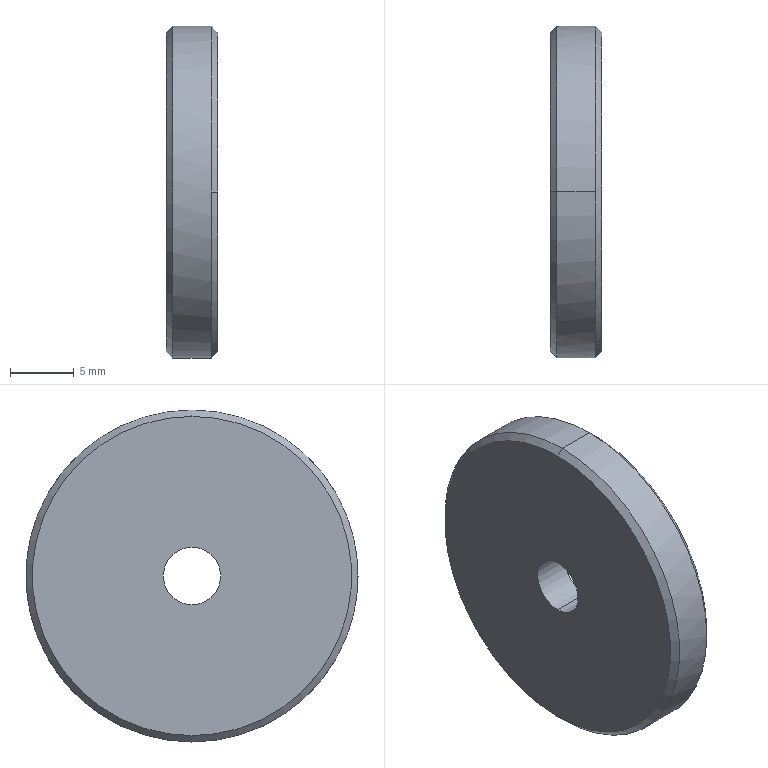Part | STEP file | locating ring 6_SUS304 | 1 solid | 13 faces | box 4 x 26 x 26 mm | volume 1943 mm3 | cylinder 6 | cone 4 | plane 3 | commonest cylinder face diameters 4.5 x2 12 x2 26 x2
STEP:
#1=CARTESIAN_POINT('',(0.,0.,0.));
#2=DIRECTION('',(0.,0.,1.));
#3=DIRECTION('',(1.,0.,0.));
#4=AXIS2_PLACEMENT_3D('',#1,#2,#3);
#5=CARTESIAN_POINT('',(0.,0.,-12.5));
#6=VERTEX_POINT('',#5);
#7=CARTESIAN_POINT('',(0.,0.,12.5));
#8=VERTEX_POINT('',#7);
#9=CARTESIAN_POINT('',(0.,0.,0.));
#10=DIRECTION('',(1.,0.,0.));
#11=DIRECTION('',(0.,0.,-1.));
#12=AXIS2_PLACEMENT_3D('',#9,#10,#11);
#13=CIRCLE('',#12,12.5);
#14=CARTESIAN_POINT('',(0.5,0.,0.));
#15=DIRECTION('',(1.,0.,0.));
#16=DIRECTION('',(0.,0.,-1.));
#17=AXIS2_PLACEMENT_3D('',#14,#15,#16);
#18=CONICAL_SURFACE('',#17,13.,0.7854);
#19=CARTESIAN_POINT('',(0.,-0.5));
#20=DIRECTION('',(1.,0.));
#21=VECTOR('',#20,1.);
#22=LINE('',#19,#21);
#23=(GEOMETRIC_REPRESENTATION_CONTEXT(2)PARAMETRIC_REPRESENTATION_CONTEXT()REPRESENTATION_CONTEXT('',''));
#24=DEFINITIONAL_REPRESENTATION('',(#22),#23);
#25=PCURVE('',#18,#24);
#26=CARTESIAN_POINT('',(0.,0.,0.));
#27=DIRECTION('',(1.,0.,0.));
#28=DIRECTION('',(0.,0.,-1.));
#29=AXIS2_PLACEMENT_3D('',#26,#27,#28);
#30=PLANE('',#29);
#31=CARTESIAN_POINT('',(0.,0.));
#32=DIRECTION('',(1.,0.));
#33=AXIS2_PLACEMENT_2D('',#31,#32);
#34=CIRCLE('',#33,12.5);
#35=(GEOMETRIC_REPRESENTATION_CONTEXT(2)PARAMETRIC_REPRESENTATION_CONTEXT()REPRESENTATION_CONTEXT('',''));
#36=DEFINITIONAL_REPRESENTATION('',(#34),#35);
#37=PCURVE('',#30,#36);
#38=SURFACE_CURVE('',#13,(#25,#37),.PCURVE_S1.);
#39=EDGE_CURVE('',#6,#8,#38,.T.);
#40=ORIENTED_EDGE('',*,*,#39,.T.);
#41=CARTESIAN_POINT('',(0.5,0.,13.));
#42=VERTEX_POINT('',#41);
#43=CARTESIAN_POINT('',(0.5,0.,13.));
#44=DIRECTION('',(0.7071,0.,0.7071));
#45=VECTOR('',#44,1.);
#46=LINE('',#43,#45);
#47=CARTESIAN_POINT('',(3.142,0.));
#48=DIRECTION('',(0.,1.));
#49=VECTOR('',#48,1.);
#50=LINE('',#47,#49);
#51=(GEOMETRIC_REPRESENTATION_CONTEXT(2)PARAMETRIC_REPRESENTATION_CONTEXT()REPRESENTATION_CONTEXT('',''));
#52=DEFINITIONAL_REPRESENTATION('',(#50),#51);
#53=PCURVE('',#18,#52);
#54=CARTESIAN_POINT('',(0.5,0.,0.));
#55=DIRECTION('',(1.,0.,0.));
#56=DIRECTION('',(0.,0.,-1.));
#57=AXIS2_PLACEMENT_3D('',#54,#55,#56);
#58=CONICAL_SURFACE('',#57,13.,0.7854);
#59=CARTESIAN_POINT('',(3.142,0.));
#60=DIRECTION('',(0.,1.));
#61=VECTOR('',#60,1.);
#62=LINE('',#59,#61);
#63=(GEOMETRIC_REPRESENTATION_CONTEXT(2)PARAMETRIC_REPRESENTATION_CONTEXT()REPRESENTATION_CONTEXT('',''));
#64=DEFINITIONAL_REPRESENTATION('',(#62),#63);
#65=PCURVE('',#58,#64);
#66=SURFACE_CURVE('',#46,(#53,#65),.PCURVE_S1.);
#67=EDGE_CURVE('',#8,#42,#66,.T.);
#68=ORIENTED_EDGE('',*,*,#67,.T.);
#69=CARTESIAN_POINT('',(0.5,0.,-13.));
#70=VERTEX_POINT('',#69);
#71=CARTESIAN_POINT('',(0.5,0.,0.));
#72=DIRECTION('',(-1.,0.,0.));
#73=DIRECTION('',(0.,0.,-1.));
#74=AXIS2_PLACEMENT_3D('',#71,#72,#73);
#75=CIRCLE('',#74,13.);
#76=CARTESIAN_POINT('',(6.283,0.));
#77=DIRECTION('',(-1.,0.));
#78=VECTOR('',#77,1.);
#79=LINE('',#76,#78);
#80=(GEOMETRIC_REPRESENTATION_CONTEXT(2)PARAMETRIC_REPRESENTATION_CONTEXT()REPRESENTATION_CONTEXT('',''));
#81=DEFINITIONAL_REPRESENTATION('',(#79),#80);
#82=PCURVE('',#18,#81);
#83=CARTESIAN_POINT('',(4.,0.,0.));
#84=DIRECTION('',(-1.,0.,0.));
#85=DIRECTION('',(0.,0.,1.));
#86=AXIS2_PLACEMENT_3D('',#83,#84,#85);
#87=CYLINDRICAL_SURFACE('',#86,13.);
#88=CARTESIAN_POINT('',(-3.142,3.5));
#89=DIRECTION('',(1.,0.));
#90=VECTOR('',#89,1.);
#91=LINE('',#88,#90);
#92=(GEOMETRIC_REPRESENTATION_CONTEXT(2)PARAMETRIC_REPRESENTATION_CONTEXT()REPRESENTATION_CONTEXT('',''));
#93=DEFINITIONAL_REPRESENTATION('',(#91),#92);
#94=PCURVE('',#87,#93);
#95=SURFACE_CURVE('',#75,(#82,#94),.PCURVE_S1.);
#96=EDGE_CURVE('',#42,#70,#95,.T.);
#97=ORIENTED_EDGE('',*,*,#96,.T.);
#98=CARTESIAN_POINT('',(0.5,0.,-13.));
#99=DIRECTION('',(0.7071,0.,-0.7071));
#100=VECTOR('',#99,1.);
#101=LINE('',#98,#100);
#102=CARTESIAN_POINT('',(0.,0.));
#103=DIRECTION('',(0.,1.));
#104=VECTOR('',#103,1.);
#105=LINE('',#102,#104);
#106=(GEOMETRIC_REPRESENTATION_CONTEXT(2)PARAMETRIC_REPRESENTATION_CONTEXT()REPRESENTATION_CONTEXT('',''));
#107=DEFINITIONAL_REPRESENTATION('',(#105),#106);
#108=PCURVE('',#18,#107);
#109=CARTESIAN_POINT('',(6.283,0.));
#110=DIRECTION('',(0.,1.));
#111=VECTOR('',#110,1.);
#112=LINE('',#109,#111);
#113=(GEOMETRIC_REPRESENTATION_CONTEXT(2)PARAMETRIC_REPRESENTATION_CONTEXT()REPRESENTATION_CONTEXT('',''));
#114=DEFINITIONAL_REPRESENTATION('',(#112),#113);
#115=PCURVE('',#58,#114);
#116=SURFACE_CURVE('',#101,(#108,#115),.PCURVE_S1.);
#117=EDGE_CURVE('',#6,#70,#116,.T.);
#118=ORIENTED_EDGE('',*,*,#117,.F.);
#119=EDGE_LOOP('',(#40,#68,#97,#118));
#120=FACE_BOUND('',#119,.T.);
#121=ADVANCED_FACE('',(#120),#18,.T.);
#122=CARTESIAN_POINT('',(3.,0.,2.25));
#123=VERTEX_POINT('',#122);
#124=CARTESIAN_POINT('',(0.,0.,2.25));
#125=VERTEX_POINT('',#124);
#126=CARTESIAN_POINT('',(4.,0.,2.25));
#127=DIRECTION('',(-1.,0.,0.));
#128=VECTOR('',#127,1.);
#129=LINE('',#126,#128);
#130=CARTESIAN_POINT('',(4.,0.,0.));
#131=DIRECTION('',(-1.,0.,0.));
#132=DIRECTION('',(0.,0.,1.));
#133=AXIS2_PLACEMENT_3D('',#130,#131,#132);
#134=CYLINDRICAL_SURFACE('',#133,2.25);
#135=CARTESIAN_POINT('',(6.283,0.));
#136=DIRECTION('',(0.,1.));
#137=VECTOR('',#136,1.);
#138=LINE('',#135,#137);
#139=(GEOMETRIC_REPRESENTATION_CONTEXT(2)PARAMETRIC_REPRESENTATION_CONTEXT()REPRESENTATION_CONTEXT('',''));
#140=DEFINITIONAL_REPRESENTATION('',(#138),#139);
#141=PCURVE('',#134,#140);
#142=CARTESIAN_POINT('',(4.,0.,0.));
#143=DIRECTION('',(-1.,0.,0.));
#144=DIRECTION('',(0.,0.,1.));
#145=AXIS2_PLACEMENT_3D('',#142,#143,#144);
#146=CYLINDRICAL_SURFACE('',#145,2.25);
#147=CARTESIAN_POINT('',(0.,0.));
#148=DIRECTION('',(0.,1.));
#149=VECTOR('',#148,1.);
#150=LINE('',#147,#149);
#151=(GEOMETRIC_REPRESENTATION_CONTEXT(2)PARAMETRIC_REPRESENTATION_CONTEXT()REPRESENTATION_CONTEXT('',''));
#152=DEFINITIONAL_REPRESENTATION('',(#150),#151);
#153=PCURVE('',#146,#152);
#154=SURFACE_CURVE('',#129,(#141,#153),.PCURVE_S1.);
#155=EDGE_CURVE('',#123,#125,#154,.T.);
#156=ORIENTED_EDGE('',*,*,#155,.T.);
#157=CARTESIAN_POINT('',(0.,0.,-2.25));
#158=VERTEX_POINT('',#157);
#159=CARTESIAN_POINT('',(0.,0.,0.));
#160=DIRECTION('',(-1.,0.,0.));
#161=DIRECTION('',(0.,0.,1.));
#162=AXIS2_PLACEMENT_3D('',#159,#160,#161);
#163=CIRCLE('',#162,2.25);
#164=CARTESIAN_POINT('',(0.,4.));
#165=DIRECTION('',(1.,0.));
#166=VECTOR('',#165,1.);
#167=LINE('',#164,#166);
#168=(GEOMETRIC_REPRESENTATION_CONTEXT(2)PARAMETRIC_REPRESENTATION_CONTEXT()REPRESENTATION_CONTEXT('',''));
#169=DEFINITIONAL_REPRESENTATION('',(#167),#168);
#170=PCURVE('',#134,#169);
#171=CARTESIAN_POINT('',(-2.25,0.));
#172=CARTESIAN_POINT('',(-2.25,3.897));
#173=CARTESIAN_POINT('',(1.125,1.949));
#174=CARTESIAN_POINT('',(4.5,0.));
#175=CARTESIAN_POINT('',(1.125,-1.949));
#176=CARTESIAN_POINT('',(-2.25,-3.897));
#177=CARTESIAN_POINT('',(-2.25,0.));
#178=(BOUNDED_CURVE()B_SPLINE_CURVE(2,(#171,#172,#173,#174,#175,#176,#177),.UNSPECIFIED.,.T.,.F.)B_SPLINE_CURVE_WITH_KNOTS((1,2,2,2,2,1),(-2.094,0.,2.094,4.189,6.283,8.378),.UNSPECIFIED.)CURVE()GEOMETRIC_REPRESENTATION_ITEM()RATIONAL_B_SPLINE_CURVE((1.,0.5,1.,0.5,1.,0.5,1.))REPRESENTATION_ITEM(''));
#179=(GEOMETRIC_REPRESENTATION_CONTEXT(2)PARAMETRIC_REPRESENTATION_CONTEXT()REPRESENTATION_CONTEXT('',''));
#180=DEFINITIONAL_REPRESENTATION('',(#178),#179);
#181=PCURVE('',#30,#180);
#182=SURFACE_CURVE('',#163,(#170,#181),.PCURVE_S1.);
#183=EDGE_CURVE('',#158,#125,#182,.T.);
#184=ORIENTED_EDGE('',*,*,#183,.F.);
#185=CARTESIAN_POINT('',(3.,0.,-2.25));
#186=VERTEX_POINT('',#185);
#187=CARTESIAN_POINT('',(4.,0.,-2.25));
#188=DIRECTION('',(-1.,0.,0.));
#189=VECTOR('',#188,1.);
#190=LINE('',#187,#189);
#191=CARTESIAN_POINT('',(3.142,0.));
#192=DIRECTION('',(0.,1.));
#193=VECTOR('',#192,1.);
#194=LINE('',#191,#193);
#195=(GEOMETRIC_REPRESENTATION_CONTEXT(2)PARAMETRIC_REPRESENTATION_CONTEXT()REPRESENTATION_CONTEXT('',''));
#196=DEFINITIONAL_REPRESENTATION('',(#194),#195);
#197=PCURVE('',#134,#196);
#198=CARTESIAN_POINT('',(3.142,0.));
#199=DIRECTION('',(0.,1.));
#200=VECTOR('',#199,1.);
#201=LINE('',#198,#200);
#202=(GEOMETRIC_REPRESENTATION_CONTEXT(2)PARAMETRIC_REPRESENTATION_CONTEXT()REPRESENTATION_CONTEXT('',''));
#203=DEFINITIONAL_REPRESENTATION('',(#201),#202);
#204=PCURVE('',#146,#203);
#205=SURFACE_CURVE('',#190,(#197,#204),.PCURVE_S1.);
#206=EDGE_CURVE('',#186,#158,#205,.T.);
#207=ORIENTED_EDGE('',*,*,#206,.F.);
#208=CARTESIAN_POINT('',(3.,0.,0.));
#209=DIRECTION('',(-1.,0.,0.));
#210=DIRECTION('',(0.,0.,1.));
#211=AXIS2_PLACEMENT_3D('',#208,#209,#210);
#212=CIRCLE('',#211,2.25);
#213=CARTESIAN_POINT('',(0.,1.));
#214=DIRECTION('',(1.,0.));
#215=VECTOR('',#214,1.);
#216=LINE('',#213,#215);
#217=(GEOMETRIC_REPRESENTATION_CONTEXT(2)PARAMETRIC_REPRESENTATION_CONTEXT()REPRESENTATION_CONTEXT('',''));
#218=DEFINITIONAL_REPRESENTATION('',(#216),#217);
#219=PCURVE('',#134,#218);
#220=CARTESIAN_POINT('',(3.,0.,0.));
#221=DIRECTION('',(1.,0.,0.));
#222=DIRECTION('',(0.,0.,-1.));
#223=AXIS2_PLACEMENT_3D('',#220,#221,#222);
#224=PLANE('',#223);
#225=CARTESIAN_POINT('',(-2.25,0.));
#226=CARTESIAN_POINT('',(-2.25,3.897));
#227=CARTESIAN_POINT('',(1.125,1.949));
#228=CARTESIAN_POINT('',(4.5,0.));
#229=CARTESIAN_POINT('',(1.125,-1.949));
#230=CARTESIAN_POINT('',(-2.25,-3.897));
#231=CARTESIAN_POINT('',(-2.25,0.));
#232=(BOUNDED_CURVE()B_SPLINE_CURVE(2,(#225,#226,#227,#228,#229,#230,#231),.UNSPECIFIED.,.T.,.F.)B_SPLINE_CURVE_WITH_KNOTS((1,2,2,2,2,1),(-2.094,0.,2.094,4.189,6.283,8.378),.UNSPECIFIED.)CURVE()GEOMETRIC_REPRESENTATION_ITEM()RATIONAL_B_SPLINE_CURVE((1.,0.5,1.,0.5,1.,0.5,1.))REPRESENTATION_ITEM(''));
#233=(GEOMETRIC_REPRESENTATION_CONTEXT(2)PARAMETRIC_REPRESENTATION_CONTEXT()REPRESENTATION_CONTEXT('',''));
#234=DEFINITIONAL_REPRESENTATION('',(#232),#233);
#235=PCURVE('',#224,#234);
#236=SURFACE_CURVE('',#212,(#219,#235),.PCURVE_S1.);
#237=EDGE_CURVE('',#186,#123,#236,.T.);
#238=ORIENTED_EDGE('',*,*,#237,.T.);
#239=EDGE_LOOP('',(#156,#184,#207,#238));
#240=FACE_BOUND('',#239,.F.);
#241=ADVANCED_FACE('',(#240),#134,.F.);
#242=CARTESIAN_POINT('',(3.5,13.,0.));
#243=VERTEX_POINT('',#242);
#244=CARTESIAN_POINT('',(3.5,0.,-13.));
#245=VERTEX_POINT('',#244);
#246=CARTESIAN_POINT('',(3.5,0.,0.));
#247=DIRECTION('',(-1.,0.,0.));
#248=DIRECTION('',(0.,0.,1.));
#249=AXIS2_PLACEMENT_3D('',#246,#247,#248);
#250=CIRCLE('',#249,13.);
#251=CARTESIAN_POINT('',(0.,0.5));
#252=DIRECTION('',(1.,0.));
#253=VECTOR('',#252,1.);
#254=LINE('',#251,#253);
#255=(GEOMETRIC_REPRESENTATION_CONTEXT(2)PARAMETRIC_REPRESENTATION_CONTEXT()REPRESENTATION_CONTEXT('',''));
#256=DEFINITIONAL_REPRESENTATION('',(#254),#255);
#257=PCURVE('',#87,#256);
#258=CARTESIAN_POINT('',(3.5,0.,0.));
#259=DIRECTION('',(-1.,0.,0.));
#260=DIRECTION('',(0.,-1.,0.));
#261=AXIS2_PLACEMENT_3D('',#258,#259,#260);
#262=CONICAL_SURFACE('',#261,13.,0.7854);
#263=CARTESIAN_POINT('',(1.571,0.));
#264=DIRECTION('',(1.,0.));
#265=VECTOR('',#264,1.);
#266=LINE('',#263,#265);
#267=(GEOMETRIC_REPRESENTATION_CONTEXT(2)PARAMETRIC_REPRESENTATION_CONTEXT()REPRESENTATION_CONTEXT('',''));
#268=DEFINITIONAL_REPRESENTATION('',(#266),#267);
#269=PCURVE('',#262,#268);
#270=SURFACE_CURVE('',#250,(#257,#269),.PCURVE_S1.);
#271=EDGE_CURVE('',#243,#245,#270,.T.);
#272=ORIENTED_EDGE('',*,*,#271,.T.);
#273=CARTESIAN_POINT('',(4.,0.,-13.));
#274=DIRECTION('',(-1.,0.,0.));
#275=VECTOR('',#274,1.);
#276=LINE('',#273,#275);
#277=CARTESIAN_POINT('',(3.142,0.));
#278=DIRECTION('',(0.,1.));
#279=VECTOR('',#278,1.);
#280=LINE('',#277,#279);
#281=(GEOMETRIC_REPRESENTATION_CONTEXT(2)PARAMETRIC_REPRESENTATION_CONTEXT()REPRESENTATION_CONTEXT('',''));
#282=DEFINITIONAL_REPRESENTATION('',(#280),#281);
#283=PCURVE('',#87,#282);
#284=CARTESIAN_POINT('',(4.,0.,0.));
#285=DIRECTION('',(-1.,0.,0.));
#286=DIRECTION('',(0.,0.,1.));
#287=AXIS2_PLACEMENT_3D('',#284,#285,#286);
#288=CYLINDRICAL_SURFACE('',#287,13.);
#289=CARTESIAN_POINT('',(3.142,0.));
#290=DIRECTION('',(0.,1.));
#291=VECTOR('',#290,1.);
#292=LINE('',#289,#291);
#293=(GEOMETRIC_REPRESENTATION_CONTEXT(2)PARAMETRIC_REPRESENTATION_CONTEXT()REPRESENTATION_CONTEXT('',''));
#294=DEFINITIONAL_REPRESENTATION('',(#292),#293);
#295=PCURVE('',#288,#294);
#296=SURFACE_CURVE('',#276,(#283,#295),.PCURVE_S1.);
#297=EDGE_CURVE('',#245,#70,#296,.T.);
#298=ORIENTED_EDGE('',*,*,#297,.T.);
#299=ORIENTED_EDGE('',*,*,#96,.F.);
#300=CARTESIAN_POINT('',(3.5,0.,13.));
#301=VERTEX_POINT('',#300);
#302=CARTESIAN_POINT('',(4.,0.,13.));
#303=DIRECTION('',(-1.,0.,0.));
#304=VECTOR('',#303,1.);
#305=LINE('',#302,#304);
#306=CARTESIAN_POINT('',(0.,0.));
#307=DIRECTION('',(0.,1.));
#308=VECTOR('',#307,1.);
#309=LINE('',#306,#308);
#310=(GEOMETRIC_REPRESENTATION_CONTEXT(2)PARAMETRIC_REPRESENTATION_CONTEXT()REPRESENTATION_CONTEXT('',''));
#311=DEFINITIONAL_REPRESENTATION('',(#309),#310);
#312=PCURVE('',#87,#311);
#313=CARTESIAN_POINT('',(6.283,0.));
#314=DIRECTION('',(0.,1.));
#315=VECTOR('',#314,1.);
#316=LINE('',#313,#315);
#317=(GEOMETRIC_REPRESENTATION_CONTEXT(2)PARAMETRIC_REPRESENTATION_CONTEXT()REPRESENTATION_CONTEXT('',''));
#318=DEFINITIONAL_REPRESENTATION('',(#316),#317);
#319=PCURVE('',#288,#318);
#320=SURFACE_CURVE('',#305,(#312,#319),.PCURVE_S1.);
#321=EDGE_CURVE('',#301,#42,#320,.T.);
#322=ORIENTED_EDGE('',*,*,#321,.F.);
#323=CARTESIAN_POINT('',(3.5,0.,0.));
#324=DIRECTION('',(-1.,0.,0.));
#325=DIRECTION('',(0.,0.,1.));
#326=AXIS2_PLACEMENT_3D('',#323,#324,#325);
#327=CIRCLE('',#326,13.);
#328=CARTESIAN_POINT('',(0.,0.5));
#329=DIRECTION('',(1.,0.));
#330=VECTOR('',#329,1.);
#331=LINE('',#328,#330);
#332=(GEOMETRIC_REPRESENTATION_CONTEXT(2)PARAMETRIC_REPRESENTATION_CONTEXT()REPRESENTATION_CONTEXT('',''));
#333=DEFINITIONAL_REPRESENTATION('',(#331),#332);
#334=PCURVE('',#87,#333);
#335=CARTESIAN_POINT('',(3.5,0.,0.));
#336=DIRECTION('',(-1.,0.,0.));
#337=DIRECTION('',(0.,-1.,0.));
#338=AXIS2_PLACEMENT_3D('',#335,#336,#337);
#339=CONICAL_SURFACE('',#338,13.,0.7854);
#340=CARTESIAN_POINT('',(1.571,0.));
#341=DIRECTION('',(1.,0.));
#342=VECTOR('',#341,1.);
#343=LINE('',#340,#342);
#344=(GEOMETRIC_REPRESENTATION_CONTEXT(2)PARAMETRIC_REPRESENTATION_CONTEXT()REPRESENTATION_CONTEXT('',''));
#345=DEFINITIONAL_REPRESENTATION('',(#343),#344);
#346=PCURVE('',#339,#345);
#347=SURFACE_CURVE('',#327,(#334,#346),.PCURVE_S1.);
#348=EDGE_CURVE('',#301,#243,#347,.T.);
#349=ORIENTED_EDGE('',*,*,#348,.T.);
#350=EDGE_LOOP('',(#272,#298,#299,#322,#349));
#351=FACE_BOUND('',#350,.T.);
#352=ADVANCED_FACE('',(#351),#87,.T.);
#353=CARTESIAN_POINT('',(4.,-12.5,0.));
#354=VERTEX_POINT('',#353);
#355=CARTESIAN_POINT('',(4.,12.5,0.));
#356=VERTEX_POINT('',#355);
#357=CARTESIAN_POINT('',(4.,0.,0.));
#358=DIRECTION('',(-1.,0.,0.));
#359=DIRECTION('',(0.,-1.,0.));
#360=AXIS2_PLACEMENT_3D('',#357,#358,#359);
#361=CIRCLE('',#360,12.5);
#362=CARTESIAN_POINT('',(0.,-0.5));
#363=DIRECTION('',(1.,0.));
#364=VECTOR('',#363,1.);
#365=LINE('',#362,#364);
#366=(GEOMETRIC_REPRESENTATION_CONTEXT(2)PARAMETRIC_REPRESENTATION_CONTEXT()REPRESENTATION_CONTEXT('',''));
#367=DEFINITIONAL_REPRESENTATION('',(#365),#366);
#368=PCURVE('',#339,#367);
#369=CARTESIAN_POINT('',(4.,0.,0.));
#370=DIRECTION('',(1.,0.,0.));
#371=DIRECTION('',(0.,0.,-1.));
#372=AXIS2_PLACEMENT_3D('',#369,#370,#371);
#373=PLANE('',#372);
#374=CARTESIAN_POINT('',(0.,-12.5));
#375=CARTESIAN_POINT('',(-21.651,-12.5));
#376=CARTESIAN_POINT('',(-10.825,6.25));
#377=CARTESIAN_POINT('',(0.,25.));
#378=CARTESIAN_POINT('',(10.825,6.25));
#379=CARTESIAN_POINT('',(21.651,-12.5));
#380=CARTESIAN_POINT('',(0.,-12.5));
#381=(BOUNDED_CURVE()B_SPLINE_CURVE(2,(#374,#375,#376,#377,#378,#379,#380),.UNSPECIFIED.,.T.,.F.)B_SPLINE_CURVE_WITH_KNOTS((1,2,2,2,2,1),(-2.094,0.,2.094,4.189,6.283,8.378),.UNSPECIFIED.)CURVE()GEOMETRIC_REPRESENTATION_ITEM()RATIONAL_B_SPLINE_CURVE((1.,0.5,1.,0.5,1.,0.5,1.))REPRESENTATION_ITEM(''));
#382=(GEOMETRIC_REPRESENTATION_CONTEXT(2)PARAMETRIC_REPRESENTATION_CONTEXT()REPRESENTATION_CONTEXT('',''));
#383=DEFINITIONAL_REPRESENTATION('',(#381),#382);
#384=PCURVE('',#373,#383);
#385=SURFACE_CURVE('',#361,(#368,#384),.PCURVE_S1.);
#386=EDGE_CURVE('',#354,#356,#385,.T.);
#387=ORIENTED_EDGE('',*,*,#386,.T.);
#388=CARTESIAN_POINT('',(3.5,13.,0.));
#389=DIRECTION('',(-0.7071,0.7071,0.));
#390=VECTOR('',#389,1.);
#391=LINE('',#388,#390);
#392=CARTESIAN_POINT('',(3.142,0.));
#393=DIRECTION('',(0.,1.));
#394=VECTOR('',#393,1.);
#395=LINE('',#392,#394);
#396=(GEOMETRIC_REPRESENTATION_CONTEXT(2)PARAMETRIC_REPRESENTATION_CONTEXT()REPRESENTATION_CONTEXT('',''));
#397=DEFINITIONAL_REPRESENTATION('',(#395),#396);
#398=PCURVE('',#339,#397);
#399=CARTESIAN_POINT('',(3.142,0.));
#400=DIRECTION('',(0.,1.));
#401=VECTOR('',#400,1.);
#402=LINE('',#399,#401);
#403=(GEOMETRIC_REPRESENTATION_CONTEXT(2)PARAMETRIC_REPRESENTATION_CONTEXT()REPRESENTATION_CONTEXT('',''));
#404=DEFINITIONAL_REPRESENTATION('',(#402),#403);
#405=PCURVE('',#262,#404);
#406=SURFACE_CURVE('',#391,(#398,#405),.PCURVE_S1.);
#407=EDGE_CURVE('',#356,#243,#406,.T.);
#408=ORIENTED_EDGE('',*,*,#407,.T.);
#409=ORIENTED_EDGE('',*,*,#348,.F.);
#410=CARTESIAN_POINT('',(3.5,-13.,0.));
#411=VERTEX_POINT('',#410);
#412=CARTESIAN_POINT('',(3.5,0.,0.));
#413=DIRECTION('',(-1.,0.,0.));
#414=DIRECTION('',(0.,0.,1.));
#415=AXIS2_PLACEMENT_3D('',#412,#413,#414);
#416=CIRCLE('',#415,13.);
#417=CARTESIAN_POINT('',(-4.712,0.));
#418=DIRECTION('',(1.,0.));
#419=VECTOR('',#418,1.);
#420=LINE('',#417,#419);
#421=(GEOMETRIC_REPRESENTATION_CONTEXT(2)PARAMETRIC_REPRESENTATION_CONTEXT()REPRESENTATION_CONTEXT('',''));
#422=DEFINITIONAL_REPRESENTATION('',(#420),#421);
#423=PCURVE('',#339,#422);
#424=CARTESIAN_POINT('',(0.,0.5));
#425=DIRECTION('',(1.,0.));
#426=VECTOR('',#425,1.);
#427=LINE('',#424,#426);
#428=(GEOMETRIC_REPRESENTATION_CONTEXT(2)PARAMETRIC_REPRESENTATION_CONTEXT()REPRESENTATION_CONTEXT('',''));
#429=DEFINITIONAL_REPRESENTATION('',(#427),#428);
#430=PCURVE('',#288,#429);
#431=SURFACE_CURVE('',#416,(#423,#430),.PCURVE_S1.);
#432=EDGE_CURVE('',#411,#301,#431,.T.);
#433=ORIENTED_EDGE('',*,*,#432,.F.);
#434=CARTESIAN_POINT('',(3.5,-13.,0.));
#435=DIRECTION('',(-0.7071,-0.7071,0.));
#436=VECTOR('',#435,1.);
#437=LINE('',#434,#436);
#438=CARTESIAN_POINT('',(0.,0.));
#439=DIRECTION('',(0.,1.));
#440=VECTOR('',#439,1.);
#441=LINE('',#438,#440);
#442=(GEOMETRIC_REPRESENTATION_CONTEXT(2)PARAMETRIC_REPRESENTATION_CONTEXT()REPRESENTATION_CONTEXT('',''));
#443=DEFINITIONAL_REPRESENTATION('',(#441),#442);
#444=PCURVE('',#339,#443);
#445=CARTESIAN_POINT('',(6.283,0.));
#446=DIRECTION('',(0.,1.));
#447=VECTOR('',#446,1.);
#448=LINE('',#445,#447);
#449=(GEOMETRIC_REPRESENTATION_CONTEXT(2)PARAMETRIC_REPRESENTATION_CONTEXT()REPRESENTATION_CONTEXT('',''));
#450=DEFINITIONAL_REPRESENTATION('',(#448),#449);
#451=PCURVE('',#262,#450);
#452=SURFACE_CURVE('',#437,(#444,#451),.PCURVE_S1.);
#453=EDGE_CURVE('',#354,#411,#452,.T.);
#454=ORIENTED_EDGE('',*,*,#453,.F.);
#455=EDGE_LOOP('',(#387,#408,#409,#433,#454));
#456=FACE_BOUND('',#455,.T.);
#457=ADVANCED_FACE('',(#456),#339,.T.);
#458=CARTESIAN_POINT('',(3.,0.,-6.));
#459=VERTEX_POINT('',#458);
#460=CARTESIAN_POINT('',(4.,0.,-6.));
#461=VERTEX_POINT('',#460);
#462=CARTESIAN_POINT('',(3.,0.,-6.));
#463=DIRECTION('',(1.,0.,0.));
#464=VECTOR('',#463,1.);
#465=LINE('',#462,#464);
#466=CARTESIAN_POINT('',(3.,0.,0.));
#467=DIRECTION('',(1.,0.,0.));
#468=DIRECTION('',(0.,0.,-1.));
#469=AXIS2_PLACEMENT_3D('',#466,#467,#468);
#470=CYLINDRICAL_SURFACE('',#469,6.);
#471=CARTESIAN_POINT('',(6.283,0.));
#472=DIRECTION('',(0.,1.));
#473=VECTOR('',#472,1.);
#474=LINE('',#471,#473);
#475=(GEOMETRIC_REPRESENTATION_CONTEXT(2)PARAMETRIC_REPRESENTATION_CONTEXT()REPRESENTATION_CONTEXT('',''));
#476=DEFINITIONAL_REPRESENTATION('',(#474),#475);
#477=PCURVE('',#470,#476);
#478=CARTESIAN_POINT('',(3.,0.,0.));
#479=DIRECTION('',(1.,0.,0.));
#480=DIRECTION('',(0.,0.,-1.));
#481=AXIS2_PLACEMENT_3D('',#478,#479,#480);
#482=CYLINDRICAL_SURFACE('',#481,6.);
#483=CARTESIAN_POINT('',(0.,0.));
#484=DIRECTION('',(0.,1.));
#485=VECTOR('',#484,1.);
#486=LINE('',#483,#485);
#487=(GEOMETRIC_REPRESENTATION_CONTEXT(2)PARAMETRIC_REPRESENTATION_CONTEXT()REPRESENTATION_CONTEXT('',''));
#488=DEFINITIONAL_REPRESENTATION('',(#486),#487);
#489=PCURVE('',#482,#488);
#490=SURFACE_CURVE('',#465,(#477,#489),.PCURVE_S1.);
#491=EDGE_CURVE('',#459,#461,#490,.T.);
#492=ORIENTED_EDGE('',*,*,#491,.T.);
#493=CARTESIAN_POINT('',(4.,0.,6.));
#494=VERTEX_POINT('',#493);
#495=CARTESIAN_POINT('',(4.,0.,0.));
#496=DIRECTION('',(-1.,0.,0.));
#497=DIRECTION('',(0.,0.,-1.));
#498=AXIS2_PLACEMENT_3D('',#495,#496,#497);
#499=CIRCLE('',#498,6.);
#500=CARTESIAN_POINT('',(6.283,1.));
#501=DIRECTION('',(-1.,0.));
#502=VECTOR('',#501,1.);
#503=LINE('',#500,#502);
#504=(GEOMETRIC_REPRESENTATION_CONTEXT(2)PARAMETRIC_REPRESENTATION_CONTEXT()REPRESENTATION_CONTEXT('',''));
#505=DEFINITIONAL_REPRESENTATION('',(#503),#504);
#506=PCURVE('',#470,#505);
#507=CARTESIAN_POINT('',(6.,0.));
#508=CARTESIAN_POINT('',(6.,-10.392));
#509=CARTESIAN_POINT('',(-3.,-5.196));
#510=CARTESIAN_POINT('',(-12.,0.));
#511=CARTESIAN_POINT('',(-3.,5.196));
#512=CARTESIAN_POINT('',(6.,10.392));
#513=CARTESIAN_POINT('',(6.,0.));
#514=(BOUNDED_CURVE()B_SPLINE_CURVE(2,(#507,#508,#509,#510,#511,#512,#513),.UNSPECIFIED.,.T.,.F.)B_SPLINE_CURVE_WITH_KNOTS((1,2,2,2,2,1),(-2.094,0.,2.094,4.189,6.283,8.378),.UNSPECIFIED.)CURVE()GEOMETRIC_REPRESENTATION_ITEM()RATIONAL_B_SPLINE_CURVE((1.,0.5,1.,0.5,1.,0.5,1.))REPRESENTATION_ITEM(''));
#515=(GEOMETRIC_REPRESENTATION_CONTEXT(2)PARAMETRIC_REPRESENTATION_CONTEXT()REPRESENTATION_CONTEXT('',''));
#516=DEFINITIONAL_REPRESENTATION('',(#514),#515);
#517=PCURVE('',#373,#516);
#518=SURFACE_CURVE('',#499,(#506,#517),.PCURVE_S1.);
#519=EDGE_CURVE('',#461,#494,#518,.T.);
#520=ORIENTED_EDGE('',*,*,#519,.T.);
#521=CARTESIAN_POINT('',(3.,0.,6.));
#522=VERTEX_POINT('',#521);
#523=CARTESIAN_POINT('',(3.,0.,6.));
#524=DIRECTION('',(1.,0.,0.));
#525=VECTOR('',#524,1.);
#526=LINE('',#523,#525);
#527=CARTESIAN_POINT('',(3.142,0.));
#528=DIRECTION('',(0.,1.));
#529=VECTOR('',#528,1.);
#530=LINE('',#527,#529);
#531=(GEOMETRIC_REPRESENTATION_CONTEXT(2)PARAMETRIC_REPRESENTATION_CONTEXT()REPRESENTATION_CONTEXT('',''));
#532=DEFINITIONAL_REPRESENTATION('',(#530),#531);
#533=PCURVE('',#470,#532);
#534=CARTESIAN_POINT('',(3.142,0.));
#535=DIRECTION('',(0.,1.));
#536=VECTOR('',#535,1.);
#537=LINE('',#534,#536);
#538=(GEOMETRIC_REPRESENTATION_CONTEXT(2)PARAMETRIC_REPRESENTATION_CONTEXT()REPRESENTATION_CONTEXT('',''));
#539=DEFINITIONAL_REPRESENTATION('',(#537),#538);
#540=PCURVE('',#482,#539);
#541=SURFACE_CURVE('',#526,(#533,#540),.PCURVE_S1.);
#542=EDGE_CURVE('',#522,#494,#541,.T.);
#543=ORIENTED_EDGE('',*,*,#542,.F.);
#544=CARTESIAN_POINT('',(3.,0.,0.));
#545=DIRECTION('',(1.,0.,0.));
#546=DIRECTION('',(0.,0.,-1.));
#547=AXIS2_PLACEMENT_3D('',#544,#545,#546);
#548=CIRCLE('',#547,6.);
#549=CARTESIAN_POINT('',(0.,0.));
#550=DIRECTION('',(1.,0.));
#551=VECTOR('',#550,1.);
#552=LINE('',#549,#551);
#553=(GEOMETRIC_REPRESENTATION_CONTEXT(2)PARAMETRIC_REPRESENTATION_CONTEXT()REPRESENTATION_CONTEXT('',''));
#554=DEFINITIONAL_REPRESENTATION('',(#552),#553);
#555=PCURVE('',#470,#554);
#556=CARTESIAN_POINT('',(0.,0.));
#557=DIRECTION('',(1.,0.));
#558=AXIS2_PLACEMENT_2D('',#556,#557);
#559=CIRCLE('',#558,6.);
#560=(GEOMETRIC_REPRESENTATION_CONTEXT(2)PARAMETRIC_REPRESENTATION_CONTEXT()REPRESENTATION_CONTEXT('',''));
#561=DEFINITIONAL_REPRESENTATION('',(#559),#560);
#562=PCURVE('',#224,#561);
#563=SURFACE_CURVE('',#548,(#555,#562),.PCURVE_S1.);
#564=EDGE_CURVE('',#522,#459,#563,.T.);
#565=ORIENTED_EDGE('',*,*,#564,.T.);
#566=EDGE_LOOP('',(#492,#520,#543,#565));
#567=FACE_BOUND('',#566,.F.);
#568=ADVANCED_FACE('',(#567),#470,.F.);
#569=ORIENTED_EDGE('',*,*,#39,.F.);
#570=CARTESIAN_POINT('',(0.,0.,0.));
#571=DIRECTION('',(1.,0.,0.));
#572=DIRECTION('',(0.,0.,-1.));
#573=AXIS2_PLACEMENT_3D('',#570,#571,#572);
#574=CIRCLE('',#573,12.5);
#575=CARTESIAN_POINT('',(0.,0.));
#576=DIRECTION('',(1.,0.));
#577=AXIS2_PLACEMENT_2D('',#575,#576);
#578=CIRCLE('',#577,12.5);
#579=(GEOMETRIC_REPRESENTATION_CONTEXT(2)PARAMETRIC_REPRESENTATION_CONTEXT()REPRESENTATION_CONTEXT('',''));
#580=DEFINITIONAL_REPRESENTATION('',(#578),#579);
#581=PCURVE('',#30,#580);
#582=CARTESIAN_POINT('',(0.,-0.5));
#583=DIRECTION('',(1.,0.));
#584=VECTOR('',#583,1.);
#585=LINE('',#582,#584);
#586=(GEOMETRIC_REPRESENTATION_CONTEXT(2)PARAMETRIC_REPRESENTATION_CONTEXT()REPRESENTATION_CONTEXT('',''));
#587=DEFINITIONAL_REPRESENTATION('',(#585),#586);
#588=PCURVE('',#58,#587);
#589=SURFACE_CURVE('',#574,(#581,#588),.PCURVE_S1.);
#590=EDGE_CURVE('',#8,#6,#589,.T.);
#591=ORIENTED_EDGE('',*,*,#590,.F.);
#592=EDGE_LOOP('',(#569,#591));
#593=FACE_BOUND('',#592,.T.);
#594=CARTESIAN_POINT('',(0.,0.,0.));
#595=DIRECTION('',(-1.,0.,0.));
#596=DIRECTION('',(0.,0.,1.));
#597=AXIS2_PLACEMENT_3D('',#594,#595,#596);
#598=CIRCLE('',#597,2.25);
#599=CARTESIAN_POINT('',(-2.25,0.));
#600=CARTESIAN_POINT('',(-2.25,3.897));
#601=CARTESIAN_POINT('',(1.125,1.949));
#602=CARTESIAN_POINT('',(4.5,0.));
#603=CARTESIAN_POINT('',(1.125,-1.949));
#604=CARTESIAN_POINT('',(-2.25,-3.897));
#605=CARTESIAN_POINT('',(-2.25,0.));
#606=(BOUNDED_CURVE()B_SPLINE_CURVE(2,(#599,#600,#601,#602,#603,#604,#605),.UNSPECIFIED.,.T.,.F.)B_SPLINE_CURVE_WITH_KNOTS((1,2,2,2,2,1),(-2.094,0.,2.094,4.189,6.283,8.378),.UNSPECIFIED.)CURVE()GEOMETRIC_REPRESENTATION_ITEM()RATIONAL_B_SPLINE_CURVE((1.,0.5,1.,0.5,1.,0.5,1.))REPRESENTATION_ITEM(''));
#607=(GEOMETRIC_REPRESENTATION_CONTEXT(2)PARAMETRIC_REPRESENTATION_CONTEXT()REPRESENTATION_CONTEXT('',''));
#608=DEFINITIONAL_REPRESENTATION('',(#606),#607);
#609=PCURVE('',#30,#608);
#610=CARTESIAN_POINT('',(0.,4.));
#611=DIRECTION('',(1.,0.));
#612=VECTOR('',#611,1.);
#613=LINE('',#610,#612);
#614=(GEOMETRIC_REPRESENTATION_CONTEXT(2)PARAMETRIC_REPRESENTATION_CONTEXT()REPRESENTATION_CONTEXT('',''));
#615=DEFINITIONAL_REPRESENTATION('',(#613),#614);
#616=PCURVE('',#146,#615);
#617=SURFACE_CURVE('',#598,(#609,#616),.PCURVE_S1.);
#618=EDGE_CURVE('',#125,#158,#617,.T.);
#619=ORIENTED_EDGE('',*,*,#618,.F.);
#620=ORIENTED_EDGE('',*,*,#183,.F.);
#621=EDGE_LOOP('',(#619,#620));
#622=FACE_BOUND('',#621,.T.);
#623=ADVANCED_FACE('',(#593,#622),#30,.F.);
#624=ORIENTED_EDGE('',*,*,#67,.F.);
#625=ORIENTED_EDGE('',*,*,#590,.T.);
#626=ORIENTED_EDGE('',*,*,#117,.T.);
#627=CARTESIAN_POINT('',(0.5,0.,0.));
#628=DIRECTION('',(-1.,0.,0.));
#629=DIRECTION('',(0.,0.,-1.));
#630=AXIS2_PLACEMENT_3D('',#627,#628,#629);
#631=CIRCLE('',#630,13.);
#632=CARTESIAN_POINT('',(6.283,0.));
#633=DIRECTION('',(-1.,0.));
#634=VECTOR('',#633,1.);
#635=LINE('',#632,#634);
#636=(GEOMETRIC_REPRESENTATION_CONTEXT(2)PARAMETRIC_REPRESENTATION_CONTEXT()REPRESENTATION_CONTEXT('',''));
#637=DEFINITIONAL_REPRESENTATION('',(#635),#636);
#638=PCURVE('',#58,#637);
#639=CARTESIAN_POINT('',(3.142,3.5));
#640=DIRECTION('',(1.,0.));
#641=VECTOR('',#640,1.);
#642=LINE('',#639,#641);
#643=(GEOMETRIC_REPRESENTATION_CONTEXT(2)PARAMETRIC_REPRESENTATION_CONTEXT()REPRESENTATION_CONTEXT('',''));
#644=DEFINITIONAL_REPRESENTATION('',(#642),#643);
#645=PCURVE('',#288,#644);
#646=SURFACE_CURVE('',#631,(#638,#645),.PCURVE_S1.);
#647=EDGE_CURVE('',#70,#42,#646,.T.);
#648=ORIENTED_EDGE('',*,*,#647,.T.);
#649=EDGE_LOOP('',(#624,#625,#626,#648));
#650=FACE_BOUND('',#649,.T.);
#651=ADVANCED_FACE('',(#650),#58,.T.);
#652=ORIENTED_EDGE('',*,*,#618,.F.);
#653=ORIENTED_EDGE('',*,*,#155,.F.);
#654=CARTESIAN_POINT('',(3.,0.,0.));
#655=DIRECTION('',(-1.,0.,0.));
#656=DIRECTION('',(0.,0.,1.));
#657=AXIS2_PLACEMENT_3D('',#654,#655,#656);
#658=CIRCLE('',#657,2.25);
#659=CARTESIAN_POINT('',(0.,1.));
#660=DIRECTION('',(1.,0.));
#661=VECTOR('',#660,1.);
#662=LINE('',#659,#661);
#663=(GEOMETRIC_REPRESENTATION_CONTEXT(2)PARAMETRIC_REPRESENTATION_CONTEXT()REPRESENTATION_CONTEXT('',''));
#664=DEFINITIONAL_REPRESENTATION('',(#662),#663);
#665=PCURVE('',#146,#664);
#666=CARTESIAN_POINT('',(-2.25,0.));
#667=CARTESIAN_POINT('',(-2.25,3.897));
#668=CARTESIAN_POINT('',(1.125,1.949));
#669=CARTESIAN_POINT('',(4.5,0.));
#670=CARTESIAN_POINT('',(1.125,-1.949));
#671=CARTESIAN_POINT('',(-2.25,-3.897));
#672=CARTESIAN_POINT('',(-2.25,0.));
#673=(BOUNDED_CURVE()B_SPLINE_CURVE(2,(#666,#667,#668,#669,#670,#671,#672),.UNSPECIFIED.,.T.,.F.)B_SPLINE_CURVE_WITH_KNOTS((1,2,2,2,2,1),(-2.094,0.,2.094,4.189,6.283,8.378),.UNSPECIFIED.)CURVE()GEOMETRIC_REPRESENTATION_ITEM()RATIONAL_B_SPLINE_CURVE((1.,0.5,1.,0.5,1.,0.5,1.))REPRESENTATION_ITEM(''));
#674=(GEOMETRIC_REPRESENTATION_CONTEXT(2)PARAMETRIC_REPRESENTATION_CONTEXT()REPRESENTATION_CONTEXT('',''));
#675=DEFINITIONAL_REPRESENTATION('',(#673),#674);
#676=PCURVE('',#224,#675);
#677=SURFACE_CURVE('',#658,(#665,#676),.PCURVE_S1.);
#678=EDGE_CURVE('',#123,#186,#677,.T.);
#679=ORIENTED_EDGE('',*,*,#678,.T.);
#680=ORIENTED_EDGE('',*,*,#206,.T.);
#681=EDGE_LOOP('',(#652,#653,#679,#680));
#682=FACE_BOUND('',#681,.F.);
#683=ADVANCED_FACE('',(#682),#146,.F.);
#684=ORIENTED_EDGE('',*,*,#297,.F.);
#685=CARTESIAN_POINT('',(3.5,0.,0.));
#686=DIRECTION('',(-1.,0.,0.));
#687=DIRECTION('',(0.,0.,1.));
#688=AXIS2_PLACEMENT_3D('',#685,#686,#687);
#689=CIRCLE('',#688,13.);
#690=CARTESIAN_POINT('',(0.,0.5));
#691=DIRECTION('',(1.,0.));
#692=VECTOR('',#691,1.);
#693=LINE('',#690,#692);
#694=(GEOMETRIC_REPRESENTATION_CONTEXT(2)PARAMETRIC_REPRESENTATION_CONTEXT()REPRESENTATION_CONTEXT('',''));
#695=DEFINITIONAL_REPRESENTATION('',(#693),#694);
#696=PCURVE('',#288,#695);
#697=CARTESIAN_POINT('',(1.571,0.));
#698=DIRECTION('',(1.,0.));
#699=VECTOR('',#698,1.);
#700=LINE('',#697,#699);
#701=(GEOMETRIC_REPRESENTATION_CONTEXT(2)PARAMETRIC_REPRESENTATION_CONTEXT()REPRESENTATION_CONTEXT('',''));
#702=DEFINITIONAL_REPRESENTATION('',(#700),#701);
#703=PCURVE('',#262,#702);
#704=SURFACE_CURVE('',#689,(#696,#703),.PCURVE_S1.);
#705=EDGE_CURVE('',#245,#411,#704,.T.);
#706=ORIENTED_EDGE('',*,*,#705,.T.);
#707=ORIENTED_EDGE('',*,*,#432,.T.);
#708=ORIENTED_EDGE('',*,*,#321,.T.);
#709=ORIENTED_EDGE('',*,*,#647,.F.);
#710=EDGE_LOOP('',(#684,#706,#707,#708,#709));
#711=FACE_BOUND('',#710,.T.);
#712=ADVANCED_FACE('',(#711),#288,.T.);
#713=ORIENTED_EDGE('',*,*,#678,.T.);
#714=ORIENTED_EDGE('',*,*,#237,.T.);
#715=EDGE_LOOP('',(#713,#714));
#716=FACE_BOUND('',#715,.T.);
#717=CARTESIAN_POINT('',(3.,0.,0.));
#718=DIRECTION('',(1.,0.,0.));
#719=DIRECTION('',(0.,0.,-1.));
#720=AXIS2_PLACEMENT_3D('',#717,#718,#719);
#721=CIRCLE('',#720,6.);
#722=CARTESIAN_POINT('',(0.,0.));
#723=DIRECTION('',(1.,0.));
#724=AXIS2_PLACEMENT_2D('',#722,#723);
#725=CIRCLE('',#724,6.);
#726=(GEOMETRIC_REPRESENTATION_CONTEXT(2)PARAMETRIC_REPRESENTATION_CONTEXT()REPRESENTATION_CONTEXT('',''));
#727=DEFINITIONAL_REPRESENTATION('',(#725),#726);
#728=PCURVE('',#224,#727);
#729=CARTESIAN_POINT('',(0.,0.));
#730=DIRECTION('',(1.,0.));
#731=VECTOR('',#730,1.);
#732=LINE('',#729,#731);
#733=(GEOMETRIC_REPRESENTATION_CONTEXT(2)PARAMETRIC_REPRESENTATION_CONTEXT()REPRESENTATION_CONTEXT('',''));
#734=DEFINITIONAL_REPRESENTATION('',(#732),#733);
#735=PCURVE('',#482,#734);
#736=SURFACE_CURVE('',#721,(#728,#735),.PCURVE_S1.);
#737=EDGE_CURVE('',#459,#522,#736,.T.);
#738=ORIENTED_EDGE('',*,*,#737,.T.);
#739=ORIENTED_EDGE('',*,*,#564,.T.);
#740=EDGE_LOOP('',(#738,#739));
#741=FACE_BOUND('',#740,.T.);
#742=ADVANCED_FACE('',(#716,#741),#224,.T.);
#743=ORIENTED_EDGE('',*,*,#407,.F.);
#744=CARTESIAN_POINT('',(4.,0.,0.));
#745=DIRECTION('',(-1.,0.,0.));
#746=DIRECTION('',(0.,-1.,0.));
#747=AXIS2_PLACEMENT_3D('',#744,#745,#746);
#748=CIRCLE('',#747,12.5);
#749=CARTESIAN_POINT('',(0.,-0.5));
#750=DIRECTION('',(1.,0.));
#751=VECTOR('',#750,1.);
#752=LINE('',#749,#751);
#753=(GEOMETRIC_REPRESENTATION_CONTEXT(2)PARAMETRIC_REPRESENTATION_CONTEXT()REPRESENTATION_CONTEXT('',''));
#754=DEFINITIONAL_REPRESENTATION('',(#752),#753);
#755=PCURVE('',#262,#754);
#756=CARTESIAN_POINT('',(0.,-12.5));
#757=CARTESIAN_POINT('',(-21.651,-12.5));
#758=CARTESIAN_POINT('',(-10.825,6.25));
#759=CARTESIAN_POINT('',(0.,25.));
#760=CARTESIAN_POINT('',(10.825,6.25));
#761=CARTESIAN_POINT('',(21.651,-12.5));
#762=CARTESIAN_POINT('',(0.,-12.5));
#763=(BOUNDED_CURVE()B_SPLINE_CURVE(2,(#756,#757,#758,#759,#760,#761,#762),.UNSPECIFIED.,.T.,.F.)B_SPLINE_CURVE_WITH_KNOTS((1,2,2,2,2,1),(-2.094,0.,2.094,4.189,6.283,8.378),.UNSPECIFIED.)CURVE()GEOMETRIC_REPRESENTATION_ITEM()RATIONAL_B_SPLINE_CURVE((1.,0.5,1.,0.5,1.,0.5,1.))REPRESENTATION_ITEM(''));
#764=(GEOMETRIC_REPRESENTATION_CONTEXT(2)PARAMETRIC_REPRESENTATION_CONTEXT()REPRESENTATION_CONTEXT('',''));
#765=DEFINITIONAL_REPRESENTATION('',(#763),#764);
#766=PCURVE('',#373,#765);
#767=SURFACE_CURVE('',#748,(#755,#766),.PCURVE_S1.);
#768=EDGE_CURVE('',#356,#354,#767,.T.);
#769=ORIENTED_EDGE('',*,*,#768,.T.);
#770=ORIENTED_EDGE('',*,*,#453,.T.);
#771=ORIENTED_EDGE('',*,*,#705,.F.);
#772=ORIENTED_EDGE('',*,*,#271,.F.);
#773=EDGE_LOOP('',(#743,#769,#770,#771,#772));
#774=FACE_BOUND('',#773,.T.);
#775=ADVANCED_FACE('',(#774),#262,.T.);
#776=CARTESIAN_POINT('',(4.,0.,0.));
#777=DIRECTION('',(-1.,0.,0.));
#778=DIRECTION('',(0.,0.,-1.));
#779=AXIS2_PLACEMENT_3D('',#776,#777,#778);
#780=CIRCLE('',#779,6.);
#781=CARTESIAN_POINT('',(6.283,1.));
#782=DIRECTION('',(-1.,0.));
#783=VECTOR('',#782,1.);
#784=LINE('',#781,#783);
#785=(GEOMETRIC_REPRESENTATION_CONTEXT(2)PARAMETRIC_REPRESENTATION_CONTEXT()REPRESENTATION_CONTEXT('',''));
#786=DEFINITIONAL_REPRESENTATION('',(#784),#785);
#787=PCURVE('',#482,#786);
#788=CARTESIAN_POINT('',(6.,0.));
#789=CARTESIAN_POINT('',(6.,-10.392));
#790=CARTESIAN_POINT('',(-3.,-5.196));
#791=CARTESIAN_POINT('',(-12.,0.));
#792=CARTESIAN_POINT('',(-3.,5.196));
#793=CARTESIAN_POINT('',(6.,10.392));
#794=CARTESIAN_POINT('',(6.,0.));
#795=(BOUNDED_CURVE()B_SPLINE_CURVE(2,(#788,#789,#790,#791,#792,#793,#794),.UNSPECIFIED.,.T.,.F.)B_SPLINE_CURVE_WITH_KNOTS((1,2,2,2,2,1),(-2.094,0.,2.094,4.189,6.283,8.378),.UNSPECIFIED.)CURVE()GEOMETRIC_REPRESENTATION_ITEM()RATIONAL_B_SPLINE_CURVE((1.,0.5,1.,0.5,1.,0.5,1.))REPRESENTATION_ITEM(''));
#796=(GEOMETRIC_REPRESENTATION_CONTEXT(2)PARAMETRIC_REPRESENTATION_CONTEXT()REPRESENTATION_CONTEXT('',''));
#797=DEFINITIONAL_REPRESENTATION('',(#795),#796);
#798=PCURVE('',#373,#797);
#799=SURFACE_CURVE('',#780,(#787,#798),.PCURVE_S1.);
#800=EDGE_CURVE('',#494,#461,#799,.T.);
#801=ORIENTED_EDGE('',*,*,#800,.T.);
#802=ORIENTED_EDGE('',*,*,#491,.F.);
#803=ORIENTED_EDGE('',*,*,#737,.T.);
#804=ORIENTED_EDGE('',*,*,#542,.T.);
#805=EDGE_LOOP('',(#801,#802,#803,#804));
#806=FACE_BOUND('',#805,.F.);
#807=ADVANCED_FACE('',(#806),#482,.F.);
#808=ORIENTED_EDGE('',*,*,#519,.T.);
#809=ORIENTED_EDGE('',*,*,#800,.T.);
#810=EDGE_LOOP('',(#808,#809));
#811=FACE_BOUND('',#810,.T.);
#812=ORIENTED_EDGE('',*,*,#386,.F.);
#813=ORIENTED_EDGE('',*,*,#768,.F.);
#814=EDGE_LOOP('',(#812,#813));
#815=FACE_BOUND('',#814,.T.);
#816=ADVANCED_FACE('',(#811,#815),#373,.T.);
#817=CLOSED_SHELL('',(#121,#241,#352,#457,#568,#623,#651,#683,#712,#742,#775,#807,#816));
#818=MANIFOLD_SOLID_BREP('',#817);
#819=(LENGTH_UNIT()NAMED_UNIT(*)SI_UNIT(.MILLI.,.METRE.));
#820=UNCERTAINTY_MEASURE_WITH_UNIT(LENGTH_MEASURE(0.0000001),#819,'','');
#821=(NAMED_UNIT(*)PLANE_ANGLE_UNIT()SI_UNIT($,.RADIAN.));
#822=(NAMED_UNIT(*)SI_UNIT($,.STERADIAN.)SOLID_ANGLE_UNIT());
#823=(GEOMETRIC_REPRESENTATION_CONTEXT(3)GLOBAL_UNCERTAINTY_ASSIGNED_CONTEXT((#820))GLOBAL_UNIT_ASSIGNED_CONTEXT((#819,#821,#822))REPRESENTATION_CONTEXT('',''));
#824=ADVANCED_BREP_SHAPE_REPRESENTATION('',(#4,#818),#823);